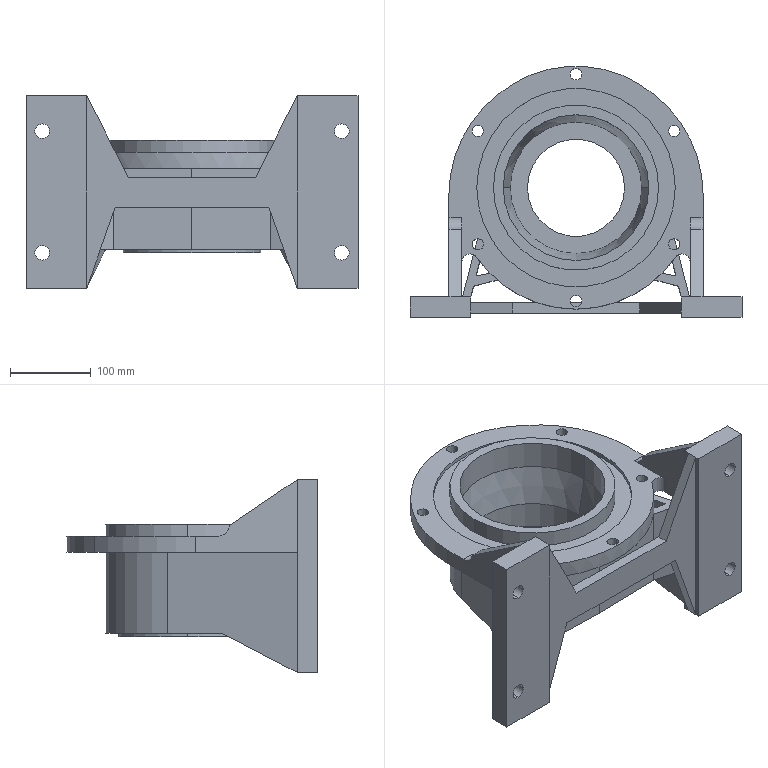Part | SolidWorks | features ICE 17, Fillet 5, Extrusion 1, MirrorPattern 1 | 1 solid | 104 faces | box 410 x 310 x 238 mm | volume 4128132 mm3 | plane 58 | cylinder 44 | cone 2 | commonest cylinder face diameters 14 x12 18 x8 20 x4 204 x4 30 x2 120 x2